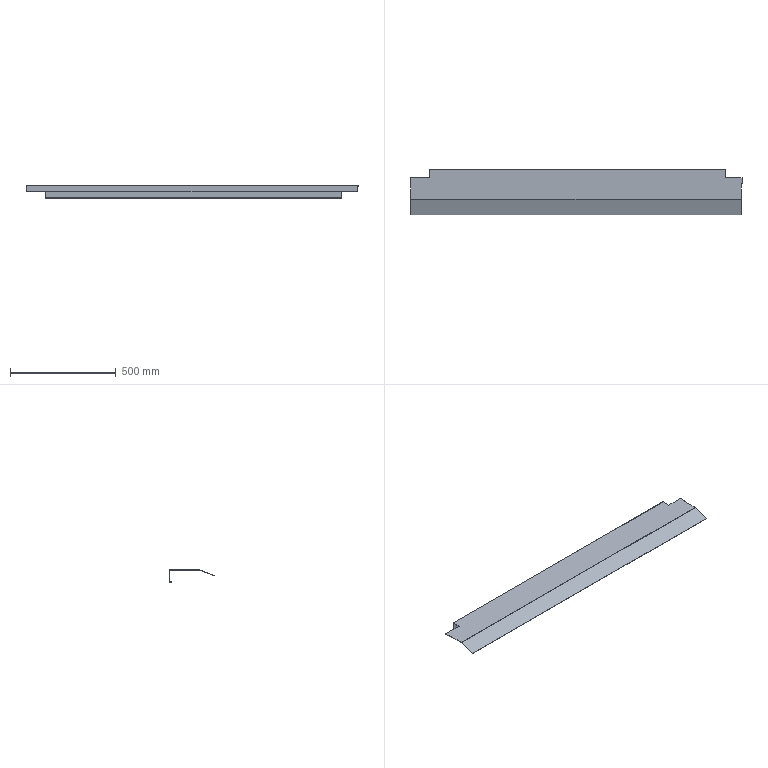Part | STEP file | Z-Direction Cover Plate | 1 solid | 26 faces | box 1571 x 215.846 x 58.382 mm | volume 647341 mm3 | plane 20 | cylinder 6 | commonest cylinder face diameters 1 x3 4 x3
STEP:
#1=CARTESIAN_POINT('',(1568.,-70.479,-1.5));
#2=VERTEX_POINT('',#1);
#3=CARTESIAN_POINT('',(1568.,0.832,-1.5));
#4=VERTEX_POINT('',#3);
#5=CARTESIAN_POINT('',(1568.,70.832,-1.5));
#6=DIRECTION('',(0.,1.,0.));
#7=VECTOR('',#6,1000.);
#8=LINE('',#5,#7);
#9=EDGE_CURVE('',#2,#4,#8,.T.);
#10=ORIENTED_EDGE('',*,*,#9,.F.);
#11=CARTESIAN_POINT('',(3.,-70.479,-1.5));
#12=VERTEX_POINT('',#11);
#13=CARTESIAN_POINT('',(1571.,-70.479,-1.5));
#14=DIRECTION('',(1.,0.,0.));
#15=VECTOR('',#14,1000.);
#16=LINE('',#13,#15);
#17=EDGE_CURVE('',#12,#2,#16,.T.);
#18=ORIENTED_EDGE('',*,*,#17,.F.);
#19=CARTESIAN_POINT('',(3.,0.832,-1.5));
#20=VERTEX_POINT('',#19);
#21=CARTESIAN_POINT('',(3.,70.832,-1.5));
#22=DIRECTION('',(0.,-1.,0.));
#23=VECTOR('',#22,1000.);
#24=LINE('',#21,#23);
#25=EDGE_CURVE('',#20,#12,#24,.T.);
#26=ORIENTED_EDGE('',*,*,#25,.F.);
#27=CARTESIAN_POINT('',(0.,0.832,-1.5));
#28=VERTEX_POINT('',#27);
#29=CARTESIAN_POINT('',(1571.,0.832,-1.5));
#30=DIRECTION('',(1.,0.,0.));
#31=VECTOR('',#30,1000.);
#32=LINE('',#29,#31);
#33=EDGE_CURVE('',#28,#20,#32,.T.);
#34=ORIENTED_EDGE('',*,*,#33,.F.);
#35=CARTESIAN_POINT('',(0.,30.832,-1.5));
#36=VERTEX_POINT('',#35);
#37=CARTESIAN_POINT('',(0.,70.832,-1.5));
#38=DIRECTION('',(0.,-1.,0.));
#39=VECTOR('',#38,1000.);
#40=LINE('',#37,#39);
#41=EDGE_CURVE('',#36,#28,#40,.T.);
#42=ORIENTED_EDGE('',*,*,#41,.F.);
#43=CARTESIAN_POINT('',(90.,30.832,-1.5));
#44=VERTEX_POINT('',#43);
#45=CARTESIAN_POINT('',(1571.,30.832,-1.5));
#46=DIRECTION('',(-1.,0.,0.));
#47=VECTOR('',#46,1000.);
#48=LINE('',#45,#47);
#49=EDGE_CURVE('',#44,#36,#48,.T.);
#50=ORIENTED_EDGE('',*,*,#49,.F.);
#51=CARTESIAN_POINT('',(90.,68.832,-1.5));
#52=VERTEX_POINT('',#51);
#53=CARTESIAN_POINT('',(90.,70.832,-1.5));
#54=DIRECTION('',(0.,-1.,0.));
#55=VECTOR('',#54,1000.);
#56=LINE('',#53,#55);
#57=EDGE_CURVE('',#52,#44,#56,.T.);
#58=ORIENTED_EDGE('',*,*,#57,.F.);
#59=CARTESIAN_POINT('',(1493.,68.832,-1.5));
#60=VERTEX_POINT('',#59);
#61=CARTESIAN_POINT('',(1571.,68.832,-1.5));
#62=DIRECTION('',(-1.,0.,0.));
#63=VECTOR('',#62,1000.);
#64=LINE('',#61,#63);
#65=EDGE_CURVE('',#60,#52,#64,.T.);
#66=ORIENTED_EDGE('',*,*,#65,.F.);
#67=CARTESIAN_POINT('',(1493.,30.832,-1.5));
#68=VERTEX_POINT('',#67);
#69=CARTESIAN_POINT('',(1493.,70.832,-1.5));
#70=DIRECTION('',(0.,1.,0.));
#71=VECTOR('',#70,1000.);
#72=LINE('',#69,#71);
#73=EDGE_CURVE('',#68,#60,#72,.T.);
#74=ORIENTED_EDGE('',*,*,#73,.F.);
#75=CARTESIAN_POINT('',(1571.,30.832,-1.5));
#76=VERTEX_POINT('',#75);
#77=CARTESIAN_POINT('',(1571.,30.832,-1.5));
#78=DIRECTION('',(-1.,0.,0.));
#79=VECTOR('',#78,1000.);
#80=LINE('',#77,#79);
#81=EDGE_CURVE('',#76,#68,#80,.T.);
#82=ORIENTED_EDGE('',*,*,#81,.F.);
#83=CARTESIAN_POINT('',(1571.,0.832,-1.5));
#84=VERTEX_POINT('',#83);
#85=CARTESIAN_POINT('',(1571.,70.832,-1.5));
#86=DIRECTION('',(0.,1.,0.));
#87=VECTOR('',#86,1000.);
#88=LINE('',#85,#87);
#89=EDGE_CURVE('',#84,#76,#88,.T.);
#90=ORIENTED_EDGE('',*,*,#89,.F.);
#91=CARTESIAN_POINT('',(1571.,0.832,-1.5));
#92=DIRECTION('',(1.,0.,0.));
#93=VECTOR('',#92,1000.);
#94=LINE('',#91,#93);
#95=EDGE_CURVE('',#4,#84,#94,.T.);
#96=ORIENTED_EDGE('',*,*,#95,.F.);
#97=EDGE_LOOP('',(#10,#18,#26,#34,#42,#50,#58,#66,#74,#82,#90,#96));
#98=FACE_OUTER_BOUND('',#97,.T.);
#99=CARTESIAN_POINT('',(1571.,70.832,-1.5));
#100=DIRECTION('',(0.,0.,1.));
#101=DIRECTION('',(0.,-1.,0.));
#102=AXIS2_PLACEMENT_3D('',#99,#100,#101);
#103=PLANE('',#102);
#104=ADVANCED_FACE('',(#98),#103,.F.);
#105=CARTESIAN_POINT('',(1568.,0.832,0.));
#106=VERTEX_POINT('',#105);
#107=CARTESIAN_POINT('',(1571.,0.832,0.));
#108=VERTEX_POINT('',#107);
#109=CARTESIAN_POINT('',(1571.,0.832,0.));
#110=DIRECTION('',(1.,0.,0.));
#111=VECTOR('',#110,1000.);
#112=LINE('',#109,#111);
#113=EDGE_CURVE('',#106,#108,#112,.T.);
#114=ORIENTED_EDGE('',*,*,#113,.F.);
#115=CARTESIAN_POINT('',(1568.,0.832,-58.382));
#116=DIRECTION('',(0.,0.,1.));
#117=VECTOR('',#116,1000.);
#118=LINE('',#115,#117);
#119=EDGE_CURVE('',#4,#106,#118,.T.);
#120=ORIENTED_EDGE('',*,*,#119,.F.);
#121=ORIENTED_EDGE('',*,*,#95,.T.);
#122=CARTESIAN_POINT('',(1571.,0.832,-58.382));
#123=DIRECTION('',(0.,0.,-1.));
#124=VECTOR('',#123,1000.);
#125=LINE('',#122,#124);
#126=EDGE_CURVE('',#108,#84,#125,.T.);
#127=ORIENTED_EDGE('',*,*,#126,.F.);
#128=EDGE_LOOP('',(#114,#120,#121,#127));
#129=FACE_OUTER_BOUND('',#128,.T.);
#130=CARTESIAN_POINT('',(1571.,0.832,-58.382));
#131=DIRECTION('',(0.,1.,0.));
#132=DIRECTION('',(-1.,0.,0.));
#133=AXIS2_PLACEMENT_3D('',#130,#131,#132);
#134=PLANE('',#133);
#135=ADVANCED_FACE('',(#129),#134,.F.);
#136=CARTESIAN_POINT('',(1568.,-70.479,0.));
#137=VERTEX_POINT('',#136);
#138=CARTESIAN_POINT('',(1568.,0.832,0.));
#139=DIRECTION('',(0.,1.,0.));
#140=VECTOR('',#139,1000.);
#141=LINE('',#138,#140);
#142=EDGE_CURVE('',#137,#106,#141,.T.);
#143=ORIENTED_EDGE('',*,*,#142,.F.);
#144=CARTESIAN_POINT('',(1568.,-71.163,-0.1206));
#145=VERTEX_POINT('',#144);
#146=CARTESIAN_POINT('',(1568.,-70.479,-2.));
#147=DIRECTION('',(-1.,0.,0.));
#148=DIRECTION('',(0.,0.,1.));
#149=AXIS2_PLACEMENT_3D('',#146,#147,#148);
#150=CIRCLE('',#149,2.);
#151=EDGE_CURVE('',#145,#137,#150,.T.);
#152=ORIENTED_EDGE('',*,*,#151,.F.);
#153=CARTESIAN_POINT('',(1568.,-145.014,-27.));
#154=VERTEX_POINT('',#153);
#155=CARTESIAN_POINT('',(1568.,-145.014,-27.));
#156=DIRECTION('',(0.,0.9397,0.342));
#157=VECTOR('',#156,1000.);
#158=LINE('',#155,#157);
#159=EDGE_CURVE('',#154,#145,#158,.T.);
#160=ORIENTED_EDGE('',*,*,#159,.F.);
#161=CARTESIAN_POINT('',(1568.,-144.501,-28.41));
#162=VERTEX_POINT('',#161);
#163=CARTESIAN_POINT('',(1568.,-144.501,-28.41));
#164=DIRECTION('',(0.,-0.342,0.9397));
#165=VECTOR('',#164,1000.);
#166=LINE('',#163,#165);
#167=EDGE_CURVE('',#162,#154,#166,.T.);
#168=ORIENTED_EDGE('',*,*,#167,.F.);
#169=CARTESIAN_POINT('',(1568.,-70.65,-1.53));
#170=VERTEX_POINT('',#169);
#171=CARTESIAN_POINT('',(1568.,-70.319,-1.41));
#172=DIRECTION('',(0.,0.9397,0.342));
#173=VECTOR('',#172,1000.);
#174=LINE('',#171,#173);
#175=EDGE_CURVE('',#162,#170,#174,.T.);
#176=ORIENTED_EDGE('',*,*,#175,.T.);
#177=CARTESIAN_POINT('',(1568.,-70.479,-2.));
#178=DIRECTION('',(-1.,0.,0.));
#179=DIRECTION('',(0.,0.,1.));
#180=AXIS2_PLACEMENT_3D('',#177,#178,#179);
#181=CIRCLE('',#180,0.5);
#182=EDGE_CURVE('',#170,#2,#181,.T.);
#183=ORIENTED_EDGE('',*,*,#182,.T.);
#184=ORIENTED_EDGE('',*,*,#9,.T.);
#185=ORIENTED_EDGE('',*,*,#119,.T.);
#186=EDGE_LOOP('',(#143,#152,#160,#168,#176,#183,#184,#185));
#187=FACE_OUTER_BOUND('',#186,.T.);
#188=CARTESIAN_POINT('',(1568.,0.832,-58.382));
#189=DIRECTION('',(-1.,0.,0.));
#190=DIRECTION('',(0.,0.,1.));
#191=AXIS2_PLACEMENT_3D('',#188,#189,#190);
#192=PLANE('',#191);
#193=ADVANCED_FACE('',(#187),#192,.F.);
#194=ORIENTED_EDGE('',*,*,#182,.F.);
#195=CARTESIAN_POINT('',(3.,-70.65,-1.53));
#196=VERTEX_POINT('',#195);
#197=CARTESIAN_POINT('',(1571.,-70.65,-1.53));
#198=DIRECTION('',(1.,0.,0.));
#199=VECTOR('',#198,1000.);
#200=LINE('',#197,#199);
#201=EDGE_CURVE('',#196,#170,#200,.T.);
#202=ORIENTED_EDGE('',*,*,#201,.F.);
#203=CARTESIAN_POINT('',(3.,-70.479,-2.));
#204=DIRECTION('',(-1.,0.,0.));
#205=DIRECTION('',(0.,0.,1.));
#206=AXIS2_PLACEMENT_3D('',#203,#204,#205);
#207=CIRCLE('',#206,0.5);
#208=EDGE_CURVE('',#196,#12,#207,.T.);
#209=ORIENTED_EDGE('',*,*,#208,.T.);
#210=ORIENTED_EDGE('',*,*,#17,.T.);
#211=EDGE_LOOP('',(#194,#202,#209,#210));
#212=FACE_OUTER_BOUND('',#211,.T.);
#213=CARTESIAN_POINT('',(1571.,-70.479,-2.));
#214=DIRECTION('',(-1.,0.,0.));
#215=DIRECTION('',(0.,0.,1.));
#216=AXIS2_PLACEMENT_3D('',#213,#214,#215);
#217=CYLINDRICAL_SURFACE('',#216,0.5);
#218=ADVANCED_FACE('',(#212),#217,.F.);
#219=ORIENTED_EDGE('',*,*,#25,.T.);
#220=ORIENTED_EDGE('',*,*,#208,.F.);
#221=CARTESIAN_POINT('',(3.,-144.501,-28.41));
#222=VERTEX_POINT('',#221);
#223=CARTESIAN_POINT('',(3.,-70.319,-1.41));
#224=DIRECTION('',(0.,-0.9397,-0.342));
#225=VECTOR('',#224,1000.);
#226=LINE('',#223,#225);
#227=EDGE_CURVE('',#196,#222,#226,.T.);
#228=ORIENTED_EDGE('',*,*,#227,.T.);
#229=CARTESIAN_POINT('',(3.,-145.014,-27.));
#230=VERTEX_POINT('',#229);
#231=CARTESIAN_POINT('',(3.,-144.501,-28.41));
#232=DIRECTION('',(0.,0.342,-0.9397));
#233=VECTOR('',#232,1000.);
#234=LINE('',#231,#233);
#235=EDGE_CURVE('',#230,#222,#234,.T.);
#236=ORIENTED_EDGE('',*,*,#235,.F.);
#237=CARTESIAN_POINT('',(3.,-71.163,-0.1206));
#238=VERTEX_POINT('',#237);
#239=CARTESIAN_POINT('',(3.,-71.163,-0.1206));
#240=DIRECTION('',(0.,-0.9397,-0.342));
#241=VECTOR('',#240,1000.);
#242=LINE('',#239,#241);
#243=EDGE_CURVE('',#238,#230,#242,.T.);
#244=ORIENTED_EDGE('',*,*,#243,.F.);
#245=CARTESIAN_POINT('',(3.,-70.479,0.));
#246=VERTEX_POINT('',#245);
#247=CARTESIAN_POINT('',(3.,-70.479,-2.));
#248=DIRECTION('',(1.,0.,0.));
#249=DIRECTION('',(0.,0.,1.));
#250=AXIS2_PLACEMENT_3D('',#247,#248,#249);
#251=CIRCLE('',#250,2.);
#252=EDGE_CURVE('',#246,#238,#251,.T.);
#253=ORIENTED_EDGE('',*,*,#252,.F.);
#254=CARTESIAN_POINT('',(3.,0.832,0.));
#255=VERTEX_POINT('',#254);
#256=CARTESIAN_POINT('',(3.,0.832,0.));
#257=DIRECTION('',(0.,-1.,0.));
#258=VECTOR('',#257,1000.);
#259=LINE('',#256,#258);
#260=EDGE_CURVE('',#255,#246,#259,.T.);
#261=ORIENTED_EDGE('',*,*,#260,.F.);
#262=CARTESIAN_POINT('',(3.,0.832,-58.382));
#263=DIRECTION('',(0.,0.,1.));
#264=VECTOR('',#263,1000.);
#265=LINE('',#262,#264);
#266=EDGE_CURVE('',#20,#255,#265,.T.);
#267=ORIENTED_EDGE('',*,*,#266,.F.);
#268=EDGE_LOOP('',(#219,#220,#228,#236,#244,#253,#261,#267));
#269=FACE_OUTER_BOUND('',#268,.T.);
#270=CARTESIAN_POINT('',(3.,0.832,-58.382));
#271=DIRECTION('',(1.,0.,0.));
#272=DIRECTION('',(0.,1.,0.));
#273=AXIS2_PLACEMENT_3D('',#270,#271,#272);
#274=PLANE('',#273);
#275=ADVANCED_FACE('',(#269),#274,.F.);
#276=CARTESIAN_POINT('',(0.,0.832,0.));
#277=VERTEX_POINT('',#276);
#278=CARTESIAN_POINT('',(0.,0.832,0.));
#279=DIRECTION('',(1.,0.,0.));
#280=VECTOR('',#279,1000.);
#281=LINE('',#278,#280);
#282=EDGE_CURVE('',#277,#255,#281,.T.);
#283=ORIENTED_EDGE('',*,*,#282,.F.);
#284=CARTESIAN_POINT('',(0.,0.832,-58.382));
#285=DIRECTION('',(0.,0.,1.));
#286=VECTOR('',#285,1000.);
#287=LINE('',#284,#286);
#288=EDGE_CURVE('',#28,#277,#287,.T.);
#289=ORIENTED_EDGE('',*,*,#288,.F.);
#290=ORIENTED_EDGE('',*,*,#33,.T.);
#291=ORIENTED_EDGE('',*,*,#266,.T.);
#292=EDGE_LOOP('',(#283,#289,#290,#291));
#293=FACE_OUTER_BOUND('',#292,.T.);
#294=CARTESIAN_POINT('',(0.,0.832,-58.382));
#295=DIRECTION('',(0.,1.,0.));
#296=DIRECTION('',(-1.,0.,0.));
#297=AXIS2_PLACEMENT_3D('',#294,#295,#296);
#298=PLANE('',#297);
#299=ADVANCED_FACE('',(#293),#298,.F.);
#300=CARTESIAN_POINT('',(0.,30.832,0.));
#301=VERTEX_POINT('',#300);
#302=CARTESIAN_POINT('',(0.,30.832,-2.));
#303=DIRECTION('',(0.,0.,-1.));
#304=VECTOR('',#303,1000.);
#305=LINE('',#302,#304);
#306=EDGE_CURVE('',#301,#36,#305,.T.);
#307=ORIENTED_EDGE('',*,*,#306,.T.);
#308=ORIENTED_EDGE('',*,*,#41,.T.);
#309=ORIENTED_EDGE('',*,*,#288,.T.);
#310=CARTESIAN_POINT('',(0.,69.332,0.));
#311=DIRECTION('',(0.,1.,0.));
#312=VECTOR('',#311,1000.);
#313=LINE('',#310,#312);
#314=EDGE_CURVE('',#277,#301,#313,.T.);
#315=ORIENTED_EDGE('',*,*,#314,.T.);
#316=EDGE_LOOP('',(#307,#308,#309,#315));
#317=FACE_OUTER_BOUND('',#316,.T.);
#318=CARTESIAN_POINT('',(0.,69.332,-2.));
#319=DIRECTION('',(-1.,0.,0.));
#320=DIRECTION('',(0.,0.,1.));
#321=AXIS2_PLACEMENT_3D('',#318,#319,#320);
#322=PLANE('',#321);
#323=ADVANCED_FACE('',(#317),#322,.T.);
#324=CARTESIAN_POINT('',(90.,30.832,0.));
#325=VERTEX_POINT('',#324);
#326=CARTESIAN_POINT('',(0.,30.832,0.));
#327=DIRECTION('',(-1.,0.,0.));
#328=VECTOR('',#327,1000.);
#329=LINE('',#326,#328);
#330=EDGE_CURVE('',#325,#301,#329,.T.);
#331=ORIENTED_EDGE('',*,*,#330,.F.);
#332=CARTESIAN_POINT('',(90.,30.832,-58.382));
#333=DIRECTION('',(0.,0.,1.));
#334=VECTOR('',#333,1000.);
#335=LINE('',#332,#334);
#336=EDGE_CURVE('',#44,#325,#335,.T.);
#337=ORIENTED_EDGE('',*,*,#336,.F.);
#338=ORIENTED_EDGE('',*,*,#49,.T.);
#339=ORIENTED_EDGE('',*,*,#306,.F.);
#340=EDGE_LOOP('',(#331,#337,#338,#339));
#341=FACE_OUTER_BOUND('',#340,.T.);
#342=CARTESIAN_POINT('',(0.,30.832,-58.382));
#343=DIRECTION('',(0.,-1.,0.));
#344=DIRECTION('',(1.,0.,0.));
#345=AXIS2_PLACEMENT_3D('',#342,#343,#344);
#346=PLANE('',#345);
#347=ADVANCED_FACE('',(#341),#346,.F.);
#348=CARTESIAN_POINT('',(90.,58.832,-58.382));
#349=VERTEX_POINT('',#348);
#350=CARTESIAN_POINT('',(90.,68.832,-58.382));
#351=VERTEX_POINT('',#350);
#352=CARTESIAN_POINT('',(90.,70.832,-58.382));
#353=DIRECTION('',(0.,1.,0.));
#354=VECTOR('',#353,1000.);
#355=LINE('',#352,#354);
#356=EDGE_CURVE('',#349,#351,#355,.T.);
#357=ORIENTED_EDGE('',*,*,#356,.F.);
#358=CARTESIAN_POINT('',(90.,58.832,-56.882));
#359=VERTEX_POINT('',#358);
#360=CARTESIAN_POINT('',(90.,58.832,-58.382));
#361=DIRECTION('',(0.,0.,-1.));
#362=VECTOR('',#361,1000.);
#363=LINE('',#360,#362);
#364=EDGE_CURVE('',#359,#349,#363,.T.);
#365=ORIENTED_EDGE('',*,*,#364,.F.);
#366=CARTESIAN_POINT('',(90.,68.832,-56.882));
#367=VERTEX_POINT('',#366);
#368=CARTESIAN_POINT('',(90.,70.832,-56.882));
#369=DIRECTION('',(0.,-1.,0.));
#370=VECTOR('',#369,1000.);
#371=LINE('',#368,#370);
#372=EDGE_CURVE('',#367,#359,#371,.T.);
#373=ORIENTED_EDGE('',*,*,#372,.F.);
#374=CARTESIAN_POINT('',(90.,69.332,-56.382));
#375=VERTEX_POINT('',#374);
#376=CARTESIAN_POINT('',(90.,68.832,-56.382));
#377=DIRECTION('',(1.,0.,0.));
#378=DIRECTION('',(0.,0.,1.));
#379=AXIS2_PLACEMENT_3D('',#376,#377,#378);
#380=CIRCLE('',#379,0.5);
#381=EDGE_CURVE('',#367,#375,#380,.T.);
#382=ORIENTED_EDGE('',*,*,#381,.T.);
#383=CARTESIAN_POINT('',(90.,69.332,-2.));
#384=VERTEX_POINT('',#383);
#385=CARTESIAN_POINT('',(90.,69.332,-58.382));
#386=DIRECTION('',(0.,0.,-1.));
#387=VECTOR('',#386,1000.);
#388=LINE('',#385,#387);
#389=EDGE_CURVE('',#384,#375,#388,.T.);
#390=ORIENTED_EDGE('',*,*,#389,.F.);
#391=CARTESIAN_POINT('',(90.,68.832,-2.));
#392=DIRECTION('',(-1.,0.,0.));
#393=DIRECTION('',(0.,0.,1.));
#394=AXIS2_PLACEMENT_3D('',#391,#392,#393);
#395=CIRCLE('',#394,0.5);
#396=EDGE_CURVE('',#52,#384,#395,.T.);
#397=ORIENTED_EDGE('',*,*,#396,.F.);
#398=ORIENTED_EDGE('',*,*,#57,.T.);
#399=ORIENTED_EDGE('',*,*,#336,.T.);
#400=CARTESIAN_POINT('',(90.,68.832,0.));
#401=VERTEX_POINT('',#400);
#402=CARTESIAN_POINT('',(90.,70.832,0.));
#403=DIRECTION('',(0.,-1.,0.));
#404=VECTOR('',#403,1000.);
#405=LINE('',#402,#404);
#406=EDGE_CURVE('',#401,#325,#405,.T.);
#407=ORIENTED_EDGE('',*,*,#406,.F.);
#408=CARTESIAN_POINT('',(90.,70.832,-2.));
#409=VERTEX_POINT('',#408);
#410=CARTESIAN_POINT('',(90.,68.832,-2.));
#411=DIRECTION('',(1.,0.,0.));
#412=DIRECTION('',(0.,0.,1.));
#413=AXIS2_PLACEMENT_3D('',#410,#411,#412);
#414=CIRCLE('',#413,2.);
#415=EDGE_CURVE('',#409,#401,#414,.T.);
#416=ORIENTED_EDGE('',*,*,#415,.F.);
#417=CARTESIAN_POINT('',(90.,70.832,-56.382));
#418=VERTEX_POINT('',#417);
#419=CARTESIAN_POINT('',(90.,70.832,-58.382));
#420=DIRECTION('',(0.,0.,1.));
#421=VECTOR('',#420,1000.);
#422=LINE('',#419,#421);
#423=EDGE_CURVE('',#418,#409,#422,.T.);
#424=ORIENTED_EDGE('',*,*,#423,.F.);
#425=CARTESIAN_POINT('',(90.,68.832,-56.382));
#426=DIRECTION('',(1.,0.,0.));
#427=DIRECTION('',(0.,0.,1.));
#428=AXIS2_PLACEMENT_3D('',#425,#426,#427);
#429=CIRCLE('',#428,2.);
#430=EDGE_CURVE('',#351,#418,#429,.T.);
#431=ORIENTED_EDGE('',*,*,#430,.F.);
#432=EDGE_LOOP('',(#357,#365,#373,#382,#390,#397,#398,#399,#407,#416,#424,#431));
#433=FACE_OUTER_BOUND('',#432,.T.);
#434=CARTESIAN_POINT('',(90.,70.832,-58.382));
#435=DIRECTION('',(1.,0.,0.));
#436=DIRECTION('',(0.,1.,0.));
#437=AXIS2_PLACEMENT_3D('',#434,#435,#436);
#438=PLANE('',#437);
#439=ADVANCED_FACE('',(#433),#438,.F.);
#440=CARTESIAN_POINT('',(1493.,69.332,-2.));
#441=VERTEX_POINT('',#440);
#442=CARTESIAN_POINT('',(1493.,68.832,-2.));
#443=DIRECTION('',(-1.,0.,0.));
#444=DIRECTION('',(0.,0.,1.));
#445=AXIS2_PLACEMENT_3D('',#442,#443,#444);
#446=CIRCLE('',#445,0.5);
#447=EDGE_CURVE('',#60,#441,#446,.T.);
#448=ORIENTED_EDGE('',*,*,#447,.F.);
#449=ORIENTED_EDGE('',*,*,#65,.T.);
#450=ORIENTED_EDGE('',*,*,#396,.T.);
#451=CARTESIAN_POINT('',(1571.,69.332,-2.));
#452=DIRECTION('',(-1.,0.,0.));
#453=VECTOR('',#452,1000.);
#454=LINE('',#451,#453);
#455=EDGE_CURVE('',#441,#384,#454,.T.);
#456=ORIENTED_EDGE('',*,*,#455,.F.);
#457=EDGE_LOOP('',(#448,#449,#450,#456));
#458=FACE_OUTER_BOUND('',#457,.T.);
#459=CARTESIAN_POINT('',(1571.,68.832,-2.));
#460=DIRECTION('',(-1.,0.,0.));
#461=DIRECTION('',(0.,0.,1.));
#462=AXIS2_PLACEMENT_3D('',#459,#460,#461);
#463=CYLINDRICAL_SURFACE('',#462,0.5);
#464=ADVANCED_FACE('',(#458),#463,.F.);
#465=CARTESIAN_POINT('',(1493.,70.832,-2.));
#466=VERTEX_POINT('',#465);
#467=CARTESIAN_POINT('',(1493.,70.832,-56.382));
#468=VERTEX_POINT('',#467);
#469=CARTESIAN_POINT('',(1493.,70.832,-58.382));
#470=DIRECTION('',(0.,0.,-1.));
#471=VECTOR('',#470,1000.);
#472=LINE('',#469,#471);
#473=EDGE_CURVE('',#466,#468,#472,.T.);
#474=ORIENTED_EDGE('',*,*,#473,.F.);
#475=CARTESIAN_POINT('',(1493.,68.832,0.));
#476=VERTEX_POINT('',#475);
#477=CARTESIAN_POINT('',(1493.,68.832,-2.));
#478=DIRECTION('',(-1.,0.,0.));
#479=DIRECTION('',(0.,0.,1.));
#480=AXIS2_PLACEMENT_3D('',#477,#478,#479);
#481=CIRCLE('',#480,2.);
#482=EDGE_CURVE('',#476,#466,#481,.T.);
#483=ORIENTED_EDGE('',*,*,#482,.F.);
#484=CARTESIAN_POINT('',(1493.,30.832,0.));
#485=VERTEX_POINT('',#484);
#486=CARTESIAN_POINT('',(1493.,70.832,0.));
#487=DIRECTION('',(0.,1.,0.));
#488=VECTOR('',#487,1000.);
#489=LINE('',#486,#488);
#490=EDGE_CURVE('',#485,#476,#489,.T.);
#491=ORIENTED_EDGE('',*,*,#490,.F.);
#492=CARTESIAN_POINT('',(1493.,30.832,-58.382));
#493=DIRECTION('',(0.,0.,1.));
#494=VECTOR('',#493,1000.);
#495=LINE('',#492,#494);
#496=EDGE_CURVE('',#68,#485,#495,.T.);
#497=ORIENTED_EDGE('',*,*,#496,.F.);
#498=ORIENTED_EDGE('',*,*,#73,.T.);
#499=ORIENTED_EDGE('',*,*,#447,.T.);
#500=CARTESIAN_POINT('',(1493.,69.332,-56.382));
#501=VERTEX_POINT('',#500);
#502=CARTESIAN_POINT('',(1493.,69.332,-58.382));
#503=DIRECTION('',(0.,0.,1.));
#504=VECTOR('',#503,1000.);
#505=LINE('',#502,#504);
#506=EDGE_CURVE('',#501,#441,#505,.T.);
#507=ORIENTED_EDGE('',*,*,#506,.F.);
#508=CARTESIAN_POINT('',(1493.,68.832,-56.882));
#509=VERTEX_POINT('',#508);
#510=CARTESIAN_POINT('',(1493.,68.832,-56.382));
#511=DIRECTION('',(-1.,0.,0.));
#512=DIRECTION('',(0.,0.,1.));
#513=AXIS2_PLACEMENT_3D('',#510,#511,#512);
#514=CIRCLE('',#513,0.5);
#515=EDGE_CURVE('',#501,#509,#514,.T.);
#516=ORIENTED_EDGE('',*,*,#515,.T.);
#517=CARTESIAN_POINT('',(1493.,58.832,-56.882));
#518=VERTEX_POINT('',#517);
#519=CARTESIAN_POINT('',(1493.,70.832,-56.882));
#520=DIRECTION('',(0.,1.,0.));
#521=VECTOR('',#520,1000.);
#522=LINE('',#519,#521);
#523=EDGE_CURVE('',#518,#509,#522,.T.);
#524=ORIENTED_EDGE('',*,*,#523,.F.);
#525=CARTESIAN_POINT('',(1493.,58.832,-58.382));
#526=VERTEX_POINT('',#525);
#527=CARTESIAN_POINT('',(1493.,58.832,-58.382));
#528=DIRECTION('',(0.,0.,1.));
#529=VECTOR('',#528,1000.);
#530=LINE('',#527,#529);
#531=EDGE_CURVE('',#526,#518,#530,.T.);
#532=ORIENTED_EDGE('',*,*,#531,.F.);
#533=CARTESIAN_POINT('',(1493.,68.832,-58.382));
#534=VERTEX_POINT('',#533);
#535=CARTESIAN_POINT('',(1493.,70.832,-58.382));
#536=DIRECTION('',(0.,-1.,0.));
#537=VECTOR('',#536,1000.);
#538=LINE('',#535,#537);
#539=EDGE_CURVE('',#534,#526,#538,.T.);
#540=ORIENTED_EDGE('',*,*,#539,.F.);
#541=CARTESIAN_POINT('',(1493.,68.832,-56.382));
#542=DIRECTION('',(-1.,0.,0.));
#543=DIRECTION('',(0.,0.,1.));
#544=AXIS2_PLACEMENT_3D('',#541,#542,#543);
#545=CIRCLE('',#544,2.);
#546=EDGE_CURVE('',#468,#534,#545,.T.);
#547=ORIENTED_EDGE('',*,*,#546,.F.);
#548=EDGE_LOOP('',(#474,#483,#491,#497,#498,#499,#507,#516,#524,#532,#540,#547));
#549=FACE_OUTER_BOUND('',#548,.T.);
#550=CARTESIAN_POINT('',(1493.,70.832,-58.382));
#551=DIRECTION('',(-1.,0.,0.));
#552=DIRECTION('',(0.,0.,1.));
#553=AXIS2_PLACEMENT_3D('',#550,#551,#552);
#554=PLANE('',#553);
#555=ADVANCED_FACE('',(#549),#554,.F.);
#556=CARTESIAN_POINT('',(1571.,30.832,0.));
#557=VERTEX_POINT('',#556);
#558=CARTESIAN_POINT('',(1571.,30.832,0.));
#559=DIRECTION('',(-1.,0.,0.));
#560=VECTOR('',#559,1000.);
#561=LINE('',#558,#560);
#562=EDGE_CURVE('',#557,#485,#561,.T.);
#563=ORIENTED_EDGE('',*,*,#562,.F.);
#564=CARTESIAN_POINT('',(1571.,30.832,-58.382));
#565=DIRECTION('',(0.,0.,1.));
#566=VECTOR('',#565,1000.);
#567=LINE('',#564,#566);
#568=EDGE_CURVE('',#76,#557,#567,.T.);
#569=ORIENTED_EDGE('',*,*,#568,.F.);
#570=ORIENTED_EDGE('',*,*,#81,.T.);
#571=ORIENTED_EDGE('',*,*,#496,.T.);
#572=EDGE_LOOP('',(#563,#569,#570,#571));
#573=FACE_OUTER_BOUND('',#572,.T.);
#574=CARTESIAN_POINT('',(1571.,30.832,-58.382));
#575=DIRECTION('',(0.,-1.,0.));
#576=DIRECTION('',(1.,0.,0.));
#577=AXIS2_PLACEMENT_3D('',#574,#575,#576);
#578=PLANE('',#577);
#579=ADVANCED_FACE('',(#573),#578,.F.);
#580=ORIENTED_EDGE('',*,*,#568,.T.);
#581=CARTESIAN_POINT('',(1571.,-70.65,0.));
#582=DIRECTION('',(0.,-1.,0.));
#583=VECTOR('',#582,1000.);
#584=LINE('',#581,#583);
#585=EDGE_CURVE('',#557,#108,#584,.T.);
#586=ORIENTED_EDGE('',*,*,#585,.T.);
#587=ORIENTED_EDGE('',*,*,#126,.T.);
#588=ORIENTED_EDGE('',*,*,#89,.T.);
#589=EDGE_LOOP('',(#580,#586,#587,#588));
#590=FACE_OUTER_BOUND('',#589,.T.);
#591=CARTESIAN_POINT('',(1571.,-70.65,-1.53));
#592=DIRECTION('',(1.,0.,0.));
#593=DIRECTION('',(0.,0.,-1.));
#594=AXIS2_PLACEMENT_3D('',#591,#592,#593);
#595=PLANE('',#594);
#596=ADVANCED_FACE('',(#590),#595,.T.);
#597=ORIENTED_EDGE('',*,*,#260,.T.);
#598=CARTESIAN_POINT('',(1571.,-70.479,0.));
#599=DIRECTION('',(1.,0.,0.));
#600=VECTOR('',#599,1000.);
#601=LINE('',#598,#600);
#602=EDGE_CURVE('',#246,#137,#601,.T.);
#603=ORIENTED_EDGE('',*,*,#602,.T.);
#604=ORIENTED_EDGE('',*,*,#142,.T.);
#605=ORIENTED_EDGE('',*,*,#113,.T.);
#606=ORIENTED_EDGE('',*,*,#585,.F.);
#607=ORIENTED_EDGE('',*,*,#562,.T.);
#608=ORIENTED_EDGE('',*,*,#490,.T.);
#609=CARTESIAN_POINT('',(1571.,68.832,0.));
#610=DIRECTION('',(-1.,0.,0.));
#611=VECTOR('',#610,1000.);
#612=LINE('',#609,#611);
#613=EDGE_CURVE('',#476,#401,#612,.T.);
#614=ORIENTED_EDGE('',*,*,#613,.T.);
#615=ORIENTED_EDGE('',*,*,#406,.T.);
#616=ORIENTED_EDGE('',*,*,#330,.T.);
#617=ORIENTED_EDGE('',*,*,#314,.F.);
#618=ORIENTED_EDGE('',*,*,#282,.T.);
#619=EDGE_LOOP('',(#597,#603,#604,#605,#606,#607,#608,#614,#615,#616,#617,#618));
#620=FACE_OUTER_BOUND('',#619,.T.);
#621=CARTESIAN_POINT('',(1571.,70.832,0.));
#622=DIRECTION('',(0.,0.,1.));
#623=DIRECTION('',(0.,-1.,0.));
#624=AXIS2_PLACEMENT_3D('',#621,#622,#623);
#625=PLANE('',#624);
#626=ADVANCED_FACE('',(#620),#625,.T.);
#627=ORIENTED_EDGE('',*,*,#175,.F.);
#628=CARTESIAN_POINT('',(1571.,-144.501,-28.41));
#629=DIRECTION('',(1.,0.,0.));
#630=VECTOR('',#629,1000.);
#631=LINE('',#628,#630);
#632=EDGE_CURVE('',#222,#162,#631,.T.);
#633=ORIENTED_EDGE('',*,*,#632,.F.);
#634=ORIENTED_EDGE('',*,*,#227,.F.);
#635=ORIENTED_EDGE('',*,*,#201,.T.);
#636=EDGE_LOOP('',(#627,#633,#634,#635));
#637=FACE_OUTER_BOUND('',#636,.T.);
#638=CARTESIAN_POINT('',(1571.,-70.319,-1.41));
#639=DIRECTION('',(0.,-0.342,0.9397));
#640=DIRECTION('',(0.,-0.9397,-0.342));
#641=AXIS2_PLACEMENT_3D('',#638,#639,#640);
#642=PLANE('',#641);
#643=ADVANCED_FACE('',(#637),#642,.F.);
#644=ORIENTED_EDGE('',*,*,#430,.T.);
#645=CARTESIAN_POINT('',(1571.,70.832,-56.382));
#646=DIRECTION('',(1.,0.,0.));
#647=VECTOR('',#646,1000.);
#648=LINE('',#645,#647);
#649=EDGE_CURVE('',#418,#468,#648,.T.);
#650=ORIENTED_EDGE('',*,*,#649,.T.);
#651=ORIENTED_EDGE('',*,*,#546,.T.);
#652=CARTESIAN_POINT('',(1571.,68.832,-58.382));
#653=DIRECTION('',(-1.,0.,0.));
#654=VECTOR('',#653,1000.);
#655=LINE('',#652,#654);
#656=EDGE_CURVE('',#534,#351,#655,.T.);
#657=ORIENTED_EDGE('',*,*,#656,.T.);
#658=EDGE_LOOP('',(#644,#650,#651,#657));
#659=FACE_OUTER_BOUND('',#658,.T.);
#660=CARTESIAN_POINT('',(1571.,68.832,-56.382));
#661=DIRECTION('',(-1.,0.,0.));
#662=DIRECTION('',(0.,0.,1.));
#663=AXIS2_PLACEMENT_3D('',#660,#661,#662);
#664=CYLINDRICAL_SURFACE('',#663,2.);
#665=ADVANCED_FACE('',(#659),#664,.T.);
#666=ORIENTED_EDGE('',*,*,#356,.T.);
#667=ORIENTED_EDGE('',*,*,#656,.F.);
#668=ORIENTED_EDGE('',*,*,#539,.T.);
#669=CARTESIAN_POINT('',(1571.,58.832,-58.382));
#670=DIRECTION('',(-1.,0.,0.));
#671=VECTOR('',#670,1000.);
#672=LINE('',#669,#671);
#673=EDGE_CURVE('',#526,#349,#672,.T.);
#674=ORIENTED_EDGE('',*,*,#673,.T.);
#675=EDGE_LOOP('',(#666,#667,#668,#674));
#676=FACE_OUTER_BOUND('',#675,.T.);
#677=CARTESIAN_POINT('',(1571.,70.832,-58.382));
#678=DIRECTION('',(0.,0.,-1.));
#679=DIRECTION('',(-1.,0.,0.));
#680=AXIS2_PLACEMENT_3D('',#677,#678,#679);
#681=PLANE('',#680);
#682=ADVANCED_FACE('',(#676),#681,.T.);
#683=ORIENTED_EDGE('',*,*,#523,.T.);
#684=CARTESIAN_POINT('',(1571.,68.832,-56.882));
#685=DIRECTION('',(1.,0.,0.));
#686=VECTOR('',#685,1000.);
#687=LINE('',#684,#686);
#688=EDGE_CURVE('',#367,#509,#687,.T.);
#689=ORIENTED_EDGE('',*,*,#688,.F.);
#690=ORIENTED_EDGE('',*,*,#372,.T.);
#691=CARTESIAN_POINT('',(1571.,58.832,-56.882));
#692=DIRECTION('',(-1.,0.,0.));
#693=VECTOR('',#692,1000.);
#694=LINE('',#691,#693);
#695=EDGE_CURVE('',#518,#359,#694,.T.);
#696=ORIENTED_EDGE('',*,*,#695,.F.);
#697=EDGE_LOOP('',(#683,#689,#690,#696));
#698=FACE_OUTER_BOUND('',#697,.T.);
#699=CARTESIAN_POINT('',(1571.,70.832,-56.882));
#700=DIRECTION('',(0.,0.,-1.));
#701=DIRECTION('',(-1.,0.,0.));
#702=AXIS2_PLACEMENT_3D('',#699,#700,#701);
#703=PLANE('',#702);
#704=ADVANCED_FACE('',(#698),#703,.F.);
#705=ORIENTED_EDGE('',*,*,#506,.T.);
#706=ORIENTED_EDGE('',*,*,#455,.T.);
#707=ORIENTED_EDGE('',*,*,#389,.T.);
#708=CARTESIAN_POINT('',(1571.,69.332,-56.382));
#709=DIRECTION('',(-1.,0.,0.));
#710=VECTOR('',#709,1000.);
#711=LINE('',#708,#710);
#712=EDGE_CURVE('',#501,#375,#711,.T.);
#713=ORIENTED_EDGE('',*,*,#712,.F.);
#714=EDGE_LOOP('',(#705,#706,#707,#713));
#715=FACE_OUTER_BOUND('',#714,.T.);
#716=CARTESIAN_POINT('',(1571.,69.332,-58.382));
#717=DIRECTION('',(0.,1.,0.));
#718=DIRECTION('',(0.,0.,1.));
#719=AXIS2_PLACEMENT_3D('',#716,#717,#718);
#720=PLANE('',#719);
#721=ADVANCED_FACE('',(#715),#720,.F.);
#722=ORIENTED_EDGE('',*,*,#415,.T.);
#723=ORIENTED_EDGE('',*,*,#613,.F.);
#724=ORIENTED_EDGE('',*,*,#482,.T.);
#725=CARTESIAN_POINT('',(1571.,70.832,-2.));
#726=DIRECTION('',(-1.,0.,0.));
#727=VECTOR('',#726,1000.);
#728=LINE('',#725,#727);
#729=EDGE_CURVE('',#466,#409,#728,.T.);
#730=ORIENTED_EDGE('',*,*,#729,.T.);
#731=EDGE_LOOP('',(#722,#723,#724,#730));
#732=FACE_OUTER_BOUND('',#731,.T.);
#733=CARTESIAN_POINT('',(1571.,68.832,-2.));
#734=DIRECTION('',(-1.,0.,0.));
#735=DIRECTION('',(0.,0.,1.));
#736=AXIS2_PLACEMENT_3D('',#733,#734,#735);
#737=CYLINDRICAL_SURFACE('',#736,2.);
#738=ADVANCED_FACE('',(#732),#737,.T.);
#739=ORIENTED_EDGE('',*,*,#423,.T.);
#740=ORIENTED_EDGE('',*,*,#729,.F.);
#741=ORIENTED_EDGE('',*,*,#473,.T.);
#742=ORIENTED_EDGE('',*,*,#649,.F.);
#743=EDGE_LOOP('',(#739,#740,#741,#742));
#744=FACE_OUTER_BOUND('',#743,.T.);
#745=CARTESIAN_POINT('',(1571.,70.832,-58.382));
#746=DIRECTION('',(0.,1.,0.));
#747=DIRECTION('',(0.,0.,1.));
#748=AXIS2_PLACEMENT_3D('',#745,#746,#747);
#749=PLANE('',#748);
#750=ADVANCED_FACE('',(#744),#749,.T.);
#751=ORIENTED_EDGE('',*,*,#252,.T.);
#752=CARTESIAN_POINT('',(1571.,-71.163,-0.1206));
#753=DIRECTION('',(1.,0.,0.));
#754=VECTOR('',#753,1000.);
#755=LINE('',#752,#754);
#756=EDGE_CURVE('',#238,#145,#755,.T.);
#757=ORIENTED_EDGE('',*,*,#756,.T.);
#758=ORIENTED_EDGE('',*,*,#151,.T.);
#759=ORIENTED_EDGE('',*,*,#602,.F.);
#760=EDGE_LOOP('',(#751,#757,#758,#759));
#761=FACE_OUTER_BOUND('',#760,.T.);
#762=CARTESIAN_POINT('',(1571.,-70.479,-2.));
#763=DIRECTION('',(-1.,0.,0.));
#764=DIRECTION('',(0.,0.,1.));
#765=AXIS2_PLACEMENT_3D('',#762,#763,#764);
#766=CYLINDRICAL_SURFACE('',#765,2.);
#767=ADVANCED_FACE('',(#761),#766,.T.);
#768=ORIENTED_EDGE('',*,*,#235,.T.);
#769=ORIENTED_EDGE('',*,*,#632,.T.);
#770=ORIENTED_EDGE('',*,*,#167,.T.);
#771=CARTESIAN_POINT('',(1571.,-145.014,-27.));
#772=DIRECTION('',(-1.,0.,0.));
#773=VECTOR('',#772,1000.);
#774=LINE('',#771,#773);
#775=EDGE_CURVE('',#154,#230,#774,.T.);
#776=ORIENTED_EDGE('',*,*,#775,.T.);
#777=EDGE_LOOP('',(#768,#769,#770,#776));
#778=FACE_OUTER_BOUND('',#777,.T.);
#779=CARTESIAN_POINT('',(1571.,-144.501,-28.41));
#780=DIRECTION('',(0.,-0.9397,-0.342));
#781=DIRECTION('',(0.,0.342,-0.9397));
#782=AXIS2_PLACEMENT_3D('',#779,#780,#781);
#783=PLANE('',#782);
#784=ADVANCED_FACE('',(#778),#783,.T.);
#785=ORIENTED_EDGE('',*,*,#364,.T.);
#786=ORIENTED_EDGE('',*,*,#673,.F.);
#787=ORIENTED_EDGE('',*,*,#531,.T.);
#788=ORIENTED_EDGE('',*,*,#695,.T.);
#789=EDGE_LOOP('',(#785,#786,#787,#788));
#790=FACE_OUTER_BOUND('',#789,.T.);
#791=CARTESIAN_POINT('',(1571.,58.832,-58.382));
#792=DIRECTION('',(0.,-1.,0.));
#793=DIRECTION('',(0.,0.,-1.));
#794=AXIS2_PLACEMENT_3D('',#791,#792,#793);
#795=PLANE('',#794);
#796=ADVANCED_FACE('',(#790),#795,.T.);
#797=ORIENTED_EDGE('',*,*,#515,.F.);
#798=ORIENTED_EDGE('',*,*,#712,.T.);
#799=ORIENTED_EDGE('',*,*,#381,.F.);
#800=ORIENTED_EDGE('',*,*,#688,.T.);
#801=EDGE_LOOP('',(#797,#798,#799,#800));
#802=FACE_OUTER_BOUND('',#801,.T.);
#803=CARTESIAN_POINT('',(1571.,68.832,-56.382));
#804=DIRECTION('',(-1.,0.,0.));
#805=DIRECTION('',(0.,0.,1.));
#806=AXIS2_PLACEMENT_3D('',#803,#804,#805);
#807=CYLINDRICAL_SURFACE('',#806,0.5);
#808=ADVANCED_FACE('',(#802),#807,.F.);
#809=ORIENTED_EDGE('',*,*,#243,.T.);
#810=ORIENTED_EDGE('',*,*,#775,.F.);
#811=ORIENTED_EDGE('',*,*,#159,.T.);
#812=ORIENTED_EDGE('',*,*,#756,.F.);
#813=EDGE_LOOP('',(#809,#810,#811,#812));
#814=FACE_OUTER_BOUND('',#813,.T.);
#815=CARTESIAN_POINT('',(1571.,-70.832,0.));
#816=DIRECTION('',(0.,-0.342,0.9397));
#817=DIRECTION('',(0.,-0.9397,-0.342));
#818=AXIS2_PLACEMENT_3D('',#815,#816,#817);
#819=PLANE('',#818);
#820=ADVANCED_FACE('',(#814),#819,.T.);
#821=CLOSED_SHELL('',(#104,#135,#193,#218,#275,#299,#323,#347,#439,#464,#555,#579,#596,#626,#643,#665,#682,#704,#721,#738,#750,#767,#784,#796,#808,#820));
#822=MANIFOLD_SOLID_BREP('',#821);
#823=CARTESIAN_POINT('',(0.,0.,0.));
#824=DIRECTION('',(0.,0.,1.));
#825=DIRECTION('',(1.,0.,0.));
#826=AXIS2_PLACEMENT_3D('',#823,#824,#825);
#827=(LENGTH_UNIT()NAMED_UNIT(*)SI_UNIT(.MILLI.,.METRE.));
#828=UNCERTAINTY_MEASURE_WITH_UNIT(LENGTH_MEASURE(0.00001),#827,'','');
#829=(NAMED_UNIT(*)PLANE_ANGLE_UNIT()SI_UNIT($,.RADIAN.));
#830=(NAMED_UNIT(*)SI_UNIT($,.STERADIAN.)SOLID_ANGLE_UNIT());
#831=(GEOMETRIC_REPRESENTATION_CONTEXT(3)GLOBAL_UNCERTAINTY_ASSIGNED_CONTEXT((#828))GLOBAL_UNIT_ASSIGNED_CONTEXT((#827,#829,#830))REPRESENTATION_CONTEXT('',''));
#832=ADVANCED_BREP_SHAPE_REPRESENTATION('',(#822,#826),#831);